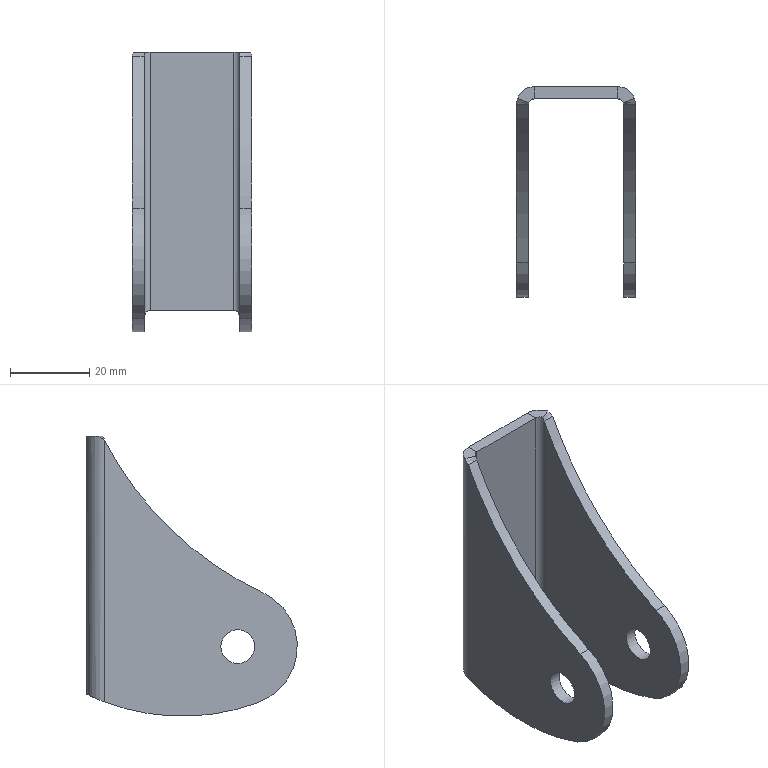Part | STEP file | 6150522 | 1 solid | 26 faces | box 30 x 53 x 70.522 mm | volume 17329 mm3 | cylinder 12 | plane 10 | spline 4 | commonest cylinder face diameters 3 x2 8.5 x2 9 x2 30 x2 110 x2 170 x2
STEP:
#1=CARTESIAN_POINT('',(-15.,-42.25,-11.5));
#2=VERTEX_POINT('',#1);
#3=CARTESIAN_POINT('',(-15.,-38.,-11.5));
#4=DIRECTION('',(-1.,0.,0.));
#5=DIRECTION('',(0.,-1.,0.));
#6=AXIS2_PLACEMENT_3D('',#3,#4,#5);
#7=CIRCLE('',#6,4.25);
#8=EDGE_CURVE('',#2,#2,#7,.T.);
#9=ORIENTED_EDGE('',*,*,#8,.F.);
#10=EDGE_LOOP('',(#9));
#11=FACE_BOUND('',#10,.T.);
#12=CARTESIAN_POINT('',(-15.,-4.5,-25.442));
#13=VERTEX_POINT('',#12);
#14=CARTESIAN_POINT('',(-15.,-4.5,40.505));
#15=VERTEX_POINT('',#14);
#16=CARTESIAN_POINT('',(-15.,-4.5,-41.5));
#17=DIRECTION('',(0.,0.,1.));
#18=VECTOR('',#17,1000.);
#19=LINE('',#16,#18);
#20=EDGE_CURVE('',#13,#15,#19,.T.);
#21=ORIENTED_EDGE('',*,*,#20,.F.);
#22=CARTESIAN_POINT('',(-15.,-43.242,-25.554));
#23=VERTEX_POINT('',#22);
#24=CARTESIAN_POINT('',(-15.,-24.02,25.978));
#25=DIRECTION('',(1.,0.,0.));
#26=DIRECTION('',(0.,-1.,0.));
#27=AXIS2_PLACEMENT_3D('',#24,#25,#26);
#28=CIRCLE('',#27,55.);
#29=EDGE_CURVE('',#23,#13,#28,.T.);
#30=ORIENTED_EDGE('',*,*,#29,.F.);
#31=CARTESIAN_POINT('',(-15.,-44.33,2.099));
#32=VERTEX_POINT('',#31);
#33=CARTESIAN_POINT('',(-15.,-38.,-11.5));
#34=DIRECTION('',(1.,0.,0.));
#35=DIRECTION('',(0.,-1.,0.));
#36=AXIS2_PLACEMENT_3D('',#33,#34,#35);
#37=CIRCLE('',#36,15.);
#38=EDGE_CURVE('',#32,#23,#37,.T.);
#39=ORIENTED_EDGE('',*,*,#38,.F.);
#40=CARTESIAN_POINT('',(-15.,-80.203,79.158));
#41=DIRECTION('',(-1.,0.,0.));
#42=DIRECTION('',(0.,-1.,0.));
#43=AXIS2_PLACEMENT_3D('',#40,#41,#42);
#44=CIRCLE('',#43,85.);
#45=EDGE_CURVE('',#15,#32,#44,.T.);
#46=ORIENTED_EDGE('',*,*,#45,.F.);
#47=EDGE_LOOP('',(#21,#30,#39,#46));
#48=FACE_OUTER_BOUND('',#47,.T.);
#49=CARTESIAN_POINT('',(-15.,0.,-41.5));
#50=DIRECTION('',(-1.,0.,0.));
#51=DIRECTION('',(0.,-1.,0.));
#52=AXIS2_PLACEMENT_3D('',#49,#50,#51);
#53=PLANE('',#52);
#54=ADVANCED_FACE('',(#11,#48),#53,.T.);
#55=CARTESIAN_POINT('',(-10.5,0.,-23.5));
#56=VERTEX_POINT('',#55);
#57=CARTESIAN_POINT('',(-10.5,0.,41.5));
#58=VERTEX_POINT('',#57);
#59=CARTESIAN_POINT('',(-10.5,0.,-41.5));
#60=DIRECTION('',(0.,0.,1.));
#61=VECTOR('',#60,1000.);
#62=LINE('',#59,#61);
#63=EDGE_CURVE('',#56,#58,#62,.T.);
#64=ORIENTED_EDGE('',*,*,#63,.F.);
#65=CARTESIAN_POINT('',(-15.,-4.5,-25.442));
#66=CARTESIAN_POINT('',(-15.,-4.21,-25.332));
#67=CARTESIAN_POINT('',(-14.972,-3.925,-25.221));
#68=CARTESIAN_POINT('',(-14.864,-3.365,-24.997));
#69=CARTESIAN_POINT('',(-14.782,-3.086,-24.884));
#70=CARTESIAN_POINT('',(-14.568,-2.554,-24.661));
#71=CARTESIAN_POINT('',(-14.436,-2.301,-24.553));
#72=CARTESIAN_POINT('',(-14.125,-1.818,-24.343));
#73=CARTESIAN_POINT('',(-13.942,-1.586,-24.24));
#74=CARTESIAN_POINT('',(-13.537,-1.166,-24.05));
#75=CARTESIAN_POINT('',(-13.315,-0.9763,-23.963));
#76=CARTESIAN_POINT('',(-12.828,-0.6378,-23.805));
#77=CARTESIAN_POINT('',(-12.562,-0.4889,-23.735));
#78=CARTESIAN_POINT('',(-12.01,-0.2503,-23.621));
#79=CARTESIAN_POINT('',(-11.722,-0.1583,-23.577));
#80=CARTESIAN_POINT('',(-11.121,-0.03245,-23.516));
#81=CARTESIAN_POINT('',(-10.811,0.,-23.5));
#82=CARTESIAN_POINT('',(-10.5,0.,-23.5));
#83=B_SPLINE_CURVE_WITH_KNOTS('',3,(#65,#66,#67,#68,#69,#70,#71,#72,#73,#74,#75,#76,#77,#78,#79,#80,#81,#82),.UNSPECIFIED.,.F.,.F.,(4,2,2,2,2,2,2,2,4),(0.,0.0009195,0.001839,0.002759,0.003678,0.004598,0.005517,0.006437,0.007356),.UNSPECIFIED.);
#84=EDGE_CURVE('',#13,#56,#83,.T.);
#85=ORIENTED_EDGE('',*,*,#84,.F.);
#86=ORIENTED_EDGE('',*,*,#20,.T.);
#87=CARTESIAN_POINT('',(-14.743,-3.,41.5));
#88=VERTEX_POINT('',#87);
#89=CARTESIAN_POINT('',(-14.743,-3.,41.5));
#90=CARTESIAN_POINT('',(-14.914,-3.484,41.173));
#91=CARTESIAN_POINT('',(-15.,-3.99,40.838));
#92=CARTESIAN_POINT('',(-15.,-4.5,40.505));
#93=B_SPLINE_CURVE_WITH_KNOTS('',3,(#89,#90,#91,#92),.UNSPECIFIED.,.F.,.F.,(4,4),(0.,0.001825),.UNSPECIFIED.);
#94=EDGE_CURVE('',#88,#15,#93,.T.);
#95=ORIENTED_EDGE('',*,*,#94,.F.);
#96=CARTESIAN_POINT('',(-10.5,-4.5,41.5));
#97=DIRECTION('',(0.,0.,1.));
#98=DIRECTION('',(-1.,0.,0.));
#99=AXIS2_PLACEMENT_3D('',#96,#97,#98);
#100=CIRCLE('',#99,4.5);
#101=EDGE_CURVE('',#58,#88,#100,.T.);
#102=ORIENTED_EDGE('',*,*,#101,.F.);
#103=EDGE_LOOP('',(#64,#85,#86,#95,#102));
#104=FACE_OUTER_BOUND('',#103,.T.);
#105=CARTESIAN_POINT('',(-10.5,-4.5,-41.5));
#106=DIRECTION('',(0.,0.,1.));
#107=DIRECTION('',(1.,0.,0.));
#108=AXIS2_PLACEMENT_3D('',#105,#106,#107);
#109=CYLINDRICAL_SURFACE('',#108,4.5);
#110=ADVANCED_FACE('',(#104),#109,.T.);
#111=CARTESIAN_POINT('',(-12.,-4.5,-25.442));
#112=VERTEX_POINT('',#111);
#113=CARTESIAN_POINT('',(-10.5,-3.,-23.5));
#114=VERTEX_POINT('',#113);
#115=CARTESIAN_POINT('',(-12.,-4.5,-25.442));
#116=CARTESIAN_POINT('',(-12.,-4.327,-25.244));
#117=CARTESIAN_POINT('',(-11.971,-4.161,-25.047));
#118=CARTESIAN_POINT('',(-11.859,-3.843,-24.652));
#119=CARTESIAN_POINT('',(-11.775,-3.689,-24.453));
#120=CARTESIAN_POINT('',(-11.545,-3.409,-24.079));
#121=CARTESIAN_POINT('',(-11.398,-3.278,-23.898));
#122=CARTESIAN_POINT('',(-11.108,-3.125,-23.68));
#123=CARTESIAN_POINT('',(-11.,-3.081,-23.617));
#124=CARTESIAN_POINT('',(-10.762,-3.018,-23.526));
#125=CARTESIAN_POINT('',(-10.633,-3.,-23.5));
#126=CARTESIAN_POINT('',(-10.5,-3.,-23.5));
#127=B_SPLINE_CURVE_WITH_KNOTS('',3,(#115,#116,#117,#118,#119,#120,#121,#122,#123,#124,#125,#126),.UNSPECIFIED.,.F.,.F.,(4,2,2,2,2,4),(0.,0.0007778,0.001556,0.002334,0.002722,0.003111),.UNSPECIFIED.);
#128=EDGE_CURVE('',#112,#114,#127,.T.);
#129=ORIENTED_EDGE('',*,*,#128,.T.);
#130=CARTESIAN_POINT('',(-10.5,-3.,41.5));
#131=VERTEX_POINT('',#130);
#132=CARTESIAN_POINT('',(-10.5,-3.,-41.5));
#133=DIRECTION('',(0.,0.,1.));
#134=VECTOR('',#133,1000.);
#135=LINE('',#132,#134);
#136=EDGE_CURVE('',#114,#131,#135,.T.);
#137=ORIENTED_EDGE('',*,*,#136,.T.);
#138=CARTESIAN_POINT('',(-11.914,-4.,41.5));
#139=VERTEX_POINT('',#138);
#140=CARTESIAN_POINT('',(-10.5,-4.5,41.5));
#141=DIRECTION('',(0.,0.,1.));
#142=DIRECTION('',(1.,0.,0.));
#143=AXIS2_PLACEMENT_3D('',#140,#141,#142);
#144=CIRCLE('',#143,1.5);
#145=EDGE_CURVE('',#131,#139,#144,.T.);
#146=ORIENTED_EDGE('',*,*,#145,.T.);
#147=CARTESIAN_POINT('',(-12.,-4.5,40.505));
#148=VERTEX_POINT('',#147);
#149=CARTESIAN_POINT('',(-11.914,-4.,41.5));
#150=CARTESIAN_POINT('',(-11.972,-4.163,41.17));
#151=CARTESIAN_POINT('',(-12.,-4.33,40.837));
#152=CARTESIAN_POINT('',(-12.,-4.5,40.505));
#153=B_SPLINE_CURVE_WITH_KNOTS('',3,(#149,#150,#151,#152),.UNSPECIFIED.,.F.,.F.,(4,4),(0.,0.001118),.UNSPECIFIED.);
#154=EDGE_CURVE('',#139,#148,#153,.T.);
#155=ORIENTED_EDGE('',*,*,#154,.T.);
#156=CARTESIAN_POINT('',(-12.,-4.5,-41.5));
#157=DIRECTION('',(0.,0.,1.));
#158=VECTOR('',#157,1000.);
#159=LINE('',#156,#158);
#160=EDGE_CURVE('',#112,#148,#159,.T.);
#161=ORIENTED_EDGE('',*,*,#160,.F.);
#162=EDGE_LOOP('',(#129,#137,#146,#155,#161));
#163=FACE_OUTER_BOUND('',#162,.T.);
#164=CARTESIAN_POINT('',(-10.5,-4.5,-41.5));
#165=DIRECTION('',(0.,0.,1.));
#166=DIRECTION('',(1.,0.,0.));
#167=AXIS2_PLACEMENT_3D('',#164,#165,#166);
#168=CYLINDRICAL_SURFACE('',#167,1.5);
#169=ADVANCED_FACE('',(#163),#168,.F.);
#170=CARTESIAN_POINT('',(-12.,-42.25,-11.5));
#171=VERTEX_POINT('',#170);
#172=CARTESIAN_POINT('',(-12.,-38.,-11.5));
#173=DIRECTION('',(-1.,0.,0.));
#174=DIRECTION('',(0.,-1.,0.));
#175=AXIS2_PLACEMENT_3D('',#172,#173,#174);
#176=CIRCLE('',#175,4.25);
#177=EDGE_CURVE('',#171,#171,#176,.T.);
#178=ORIENTED_EDGE('',*,*,#177,.T.);
#179=EDGE_LOOP('',(#178));
#180=FACE_BOUND('',#179,.T.);
#181=CARTESIAN_POINT('',(-12.,-43.242,-25.554));
#182=VERTEX_POINT('',#181);
#183=CARTESIAN_POINT('',(-12.,-24.02,25.978));
#184=DIRECTION('',(1.,0.,0.));
#185=DIRECTION('',(0.,-1.,0.));
#186=AXIS2_PLACEMENT_3D('',#183,#184,#185);
#187=CIRCLE('',#186,55.);
#188=EDGE_CURVE('',#182,#112,#187,.T.);
#189=ORIENTED_EDGE('',*,*,#188,.T.);
#190=ORIENTED_EDGE('',*,*,#160,.T.);
#191=CARTESIAN_POINT('',(-12.,-44.33,2.099));
#192=VERTEX_POINT('',#191);
#193=CARTESIAN_POINT('',(-12.,-80.203,79.158));
#194=DIRECTION('',(-1.,0.,0.));
#195=DIRECTION('',(0.,-1.,0.));
#196=AXIS2_PLACEMENT_3D('',#193,#194,#195);
#197=CIRCLE('',#196,85.);
#198=EDGE_CURVE('',#148,#192,#197,.T.);
#199=ORIENTED_EDGE('',*,*,#198,.T.);
#200=CARTESIAN_POINT('',(-12.,-38.,-11.5));
#201=DIRECTION('',(1.,0.,0.));
#202=DIRECTION('',(0.,-1.,0.));
#203=AXIS2_PLACEMENT_3D('',#200,#201,#202);
#204=CIRCLE('',#203,15.);
#205=EDGE_CURVE('',#192,#182,#204,.T.);
#206=ORIENTED_EDGE('',*,*,#205,.T.);
#207=EDGE_LOOP('',(#189,#190,#199,#206));
#208=FACE_OUTER_BOUND('',#207,.T.);
#209=CARTESIAN_POINT('',(-12.,0.,-41.5));
#210=DIRECTION('',(-1.,0.,0.));
#211=DIRECTION('',(0.,-1.,0.));
#212=AXIS2_PLACEMENT_3D('',#209,#210,#211);
#213=PLANE('',#212);
#214=ADVANCED_FACE('',(#180,#208),#213,.F.);
#215=CARTESIAN_POINT('',(15.,-4.5,-25.442));
#216=VERTEX_POINT('',#215);
#217=CARTESIAN_POINT('',(15.,-4.5,40.505));
#218=VERTEX_POINT('',#217);
#219=CARTESIAN_POINT('',(15.,-4.5,-41.5));
#220=DIRECTION('',(0.,0.,1.));
#221=VECTOR('',#220,1000.);
#222=LINE('',#219,#221);
#223=EDGE_CURVE('',#216,#218,#222,.T.);
#224=ORIENTED_EDGE('',*,*,#223,.F.);
#225=CARTESIAN_POINT('',(10.5,0.,-23.5));
#226=VERTEX_POINT('',#225);
#227=CARTESIAN_POINT('',(10.5,0.,-23.5));
#228=CARTESIAN_POINT('',(10.81,0.,-23.5));
#229=CARTESIAN_POINT('',(11.114,-0.03178,-23.515));
#230=CARTESIAN_POINT('',(11.56,-0.124,-23.56));
#231=CARTESIAN_POINT('',(11.707,-0.1622,-23.579));
#232=CARTESIAN_POINT('',(11.998,-0.2538,-23.623));
#233=CARTESIAN_POINT('',(12.142,-0.3074,-23.648));
#234=CARTESIAN_POINT('',(12.558,-0.4869,-23.734));
#235=CARTESIAN_POINT('',(12.819,-0.6322,-23.802));
#236=CARTESIAN_POINT('',(13.309,-0.9719,-23.961));
#237=CARTESIAN_POINT('',(13.535,-1.165,-24.049));
#238=CARTESIAN_POINT('',(13.94,-1.584,-24.239));
#239=CARTESIAN_POINT('',(14.122,-1.814,-24.341));
#240=CARTESIAN_POINT('',(14.436,-2.3,-24.553));
#241=CARTESIAN_POINT('',(14.568,-2.554,-24.661));
#242=CARTESIAN_POINT('',(14.781,-3.084,-24.883));
#243=CARTESIAN_POINT('',(14.863,-3.362,-24.996));
#244=CARTESIAN_POINT('',(14.972,-3.925,-25.221));
#245=CARTESIAN_POINT('',(15.,-4.21,-25.332));
#246=CARTESIAN_POINT('',(15.,-4.5,-25.442));
#247=B_SPLINE_CURVE_WITH_KNOTS('',3,(#227,#228,#229,#230,#231,#232,#233,#234,#235,#236,#237,#238,#239,#240,#241,#242,#243,#244,#245,#246),.UNSPECIFIED.,.F.,.F.,(4,2,2,2,2,2,2,2,2,4),(0.,0.0009144,0.001372,0.001829,0.002743,0.003657,0.004572,0.005486,0.006401,0.007315),.UNSPECIFIED.);
#248=EDGE_CURVE('',#226,#216,#247,.T.);
#249=ORIENTED_EDGE('',*,*,#248,.F.);
#250=CARTESIAN_POINT('',(10.5,0.,41.5));
#251=VERTEX_POINT('',#250);
#252=CARTESIAN_POINT('',(10.5,0.,-41.5));
#253=DIRECTION('',(0.,0.,1.));
#254=VECTOR('',#253,1000.);
#255=LINE('',#252,#254);
#256=EDGE_CURVE('',#226,#251,#255,.T.);
#257=ORIENTED_EDGE('',*,*,#256,.T.);
#258=CARTESIAN_POINT('',(14.743,-3.,41.5));
#259=VERTEX_POINT('',#258);
#260=CARTESIAN_POINT('',(10.5,-4.5,41.5));
#261=DIRECTION('',(0.,0.,1.));
#262=DIRECTION('',(-1.,0.,0.));
#263=AXIS2_PLACEMENT_3D('',#260,#261,#262);
#264=CIRCLE('',#263,4.5);
#265=EDGE_CURVE('',#259,#251,#264,.T.);
#266=ORIENTED_EDGE('',*,*,#265,.F.);
#267=CARTESIAN_POINT('',(15.,-4.5,40.505));
#268=CARTESIAN_POINT('',(15.,-3.99,40.838));
#269=CARTESIAN_POINT('',(14.914,-3.484,41.173));
#270=CARTESIAN_POINT('',(14.743,-3.,41.5));
#271=B_SPLINE_CURVE_WITH_KNOTS('',3,(#267,#268,#269,#270),.UNSPECIFIED.,.F.,.F.,(4,4),(0.,0.001825),.UNSPECIFIED.);
#272=EDGE_CURVE('',#218,#259,#271,.T.);
#273=ORIENTED_EDGE('',*,*,#272,.F.);
#274=EDGE_LOOP('',(#224,#249,#257,#266,#273));
#275=FACE_OUTER_BOUND('',#274,.T.);
#276=CARTESIAN_POINT('',(10.5,-4.5,-41.5));
#277=DIRECTION('',(0.,0.,1.));
#278=DIRECTION('',(1.,0.,0.));
#279=AXIS2_PLACEMENT_3D('',#276,#277,#278);
#280=CYLINDRICAL_SURFACE('',#279,4.5);
#281=ADVANCED_FACE('',(#275),#280,.T.);
#282=CARTESIAN_POINT('',(15.,-33.75,-11.5));
#283=VERTEX_POINT('',#282);
#284=CARTESIAN_POINT('',(15.,-38.,-11.5));
#285=DIRECTION('',(1.,0.,0.));
#286=DIRECTION('',(0.,1.,0.));
#287=AXIS2_PLACEMENT_3D('',#284,#285,#286);
#288=CIRCLE('',#287,4.25);
#289=EDGE_CURVE('',#283,#283,#288,.T.);
#290=ORIENTED_EDGE('',*,*,#289,.F.);
#291=EDGE_LOOP('',(#290));
#292=FACE_BOUND('',#291,.T.);
#293=CARTESIAN_POINT('',(15.,-43.242,-25.554));
#294=VERTEX_POINT('',#293);
#295=CARTESIAN_POINT('',(15.,-44.33,2.099));
#296=VERTEX_POINT('',#295);
#297=CARTESIAN_POINT('',(15.,-38.,-11.5));
#298=DIRECTION('',(-1.,0.,0.));
#299=DIRECTION('',(0.,1.,0.));
#300=AXIS2_PLACEMENT_3D('',#297,#298,#299);
#301=CIRCLE('',#300,15.);
#302=EDGE_CURVE('',#294,#296,#301,.T.);
#303=ORIENTED_EDGE('',*,*,#302,.F.);
#304=CARTESIAN_POINT('',(15.,-24.02,25.978));
#305=DIRECTION('',(-1.,0.,0.));
#306=DIRECTION('',(0.,1.,0.));
#307=AXIS2_PLACEMENT_3D('',#304,#305,#306);
#308=CIRCLE('',#307,55.);
#309=EDGE_CURVE('',#216,#294,#308,.T.);
#310=ORIENTED_EDGE('',*,*,#309,.F.);
#311=ORIENTED_EDGE('',*,*,#223,.T.);
#312=CARTESIAN_POINT('',(15.,-80.203,79.158));
#313=DIRECTION('',(1.,0.,0.));
#314=DIRECTION('',(0.,1.,0.));
#315=AXIS2_PLACEMENT_3D('',#312,#313,#314);
#316=CIRCLE('',#315,85.);
#317=EDGE_CURVE('',#296,#218,#316,.T.);
#318=ORIENTED_EDGE('',*,*,#317,.F.);
#319=EDGE_LOOP('',(#303,#310,#311,#318));
#320=FACE_OUTER_BOUND('',#319,.T.);
#321=CARTESIAN_POINT('',(15.,0.,-41.5));
#322=DIRECTION('',(1.,0.,0.));
#323=DIRECTION('',(0.,1.,0.));
#324=AXIS2_PLACEMENT_3D('',#321,#322,#323);
#325=PLANE('',#324);
#326=ADVANCED_FACE('',(#292,#320),#325,.T.);
#327=CARTESIAN_POINT('',(12.,-33.75,-11.5));
#328=VERTEX_POINT('',#327);
#329=CARTESIAN_POINT('',(12.,-38.,-11.5));
#330=DIRECTION('',(1.,0.,0.));
#331=DIRECTION('',(0.,1.,0.));
#332=AXIS2_PLACEMENT_3D('',#329,#330,#331);
#333=CIRCLE('',#332,4.25);
#334=EDGE_CURVE('',#328,#328,#333,.T.);
#335=ORIENTED_EDGE('',*,*,#334,.T.);
#336=EDGE_LOOP('',(#335));
#337=FACE_BOUND('',#336,.T.);
#338=CARTESIAN_POINT('',(12.,-4.5,-25.442));
#339=VERTEX_POINT('',#338);
#340=CARTESIAN_POINT('',(12.,-43.242,-25.554));
#341=VERTEX_POINT('',#340);
#342=CARTESIAN_POINT('',(12.,-24.02,25.978));
#343=DIRECTION('',(-1.,0.,0.));
#344=DIRECTION('',(0.,1.,0.));
#345=AXIS2_PLACEMENT_3D('',#342,#343,#344);
#346=CIRCLE('',#345,55.);
#347=EDGE_CURVE('',#339,#341,#346,.T.);
#348=ORIENTED_EDGE('',*,*,#347,.T.);
#349=CARTESIAN_POINT('',(12.,-44.33,2.099));
#350=VERTEX_POINT('',#349);
#351=CARTESIAN_POINT('',(12.,-38.,-11.5));
#352=DIRECTION('',(-1.,0.,0.));
#353=DIRECTION('',(0.,1.,0.));
#354=AXIS2_PLACEMENT_3D('',#351,#352,#353);
#355=CIRCLE('',#354,15.);
#356=EDGE_CURVE('',#341,#350,#355,.T.);
#357=ORIENTED_EDGE('',*,*,#356,.T.);
#358=CARTESIAN_POINT('',(12.,-4.5,40.505));
#359=VERTEX_POINT('',#358);
#360=CARTESIAN_POINT('',(12.,-80.203,79.158));
#361=DIRECTION('',(1.,0.,0.));
#362=DIRECTION('',(0.,1.,0.));
#363=AXIS2_PLACEMENT_3D('',#360,#361,#362);
#364=CIRCLE('',#363,85.);
#365=EDGE_CURVE('',#350,#359,#364,.T.);
#366=ORIENTED_EDGE('',*,*,#365,.T.);
#367=CARTESIAN_POINT('',(12.,-4.5,-41.5));
#368=DIRECTION('',(0.,0.,1.));
#369=VECTOR('',#368,1000.);
#370=LINE('',#367,#369);
#371=EDGE_CURVE('',#339,#359,#370,.T.);
#372=ORIENTED_EDGE('',*,*,#371,.F.);
#373=EDGE_LOOP('',(#348,#357,#366,#372));
#374=FACE_OUTER_BOUND('',#373,.T.);
#375=CARTESIAN_POINT('',(12.,0.,-41.5));
#376=DIRECTION('',(1.,0.,0.));
#377=DIRECTION('',(0.,1.,0.));
#378=AXIS2_PLACEMENT_3D('',#375,#376,#377);
#379=PLANE('',#378);
#380=ADVANCED_FACE('',(#337,#374),#379,.F.);
#381=CARTESIAN_POINT('',(10.5,-3.,-23.5));
#382=VERTEX_POINT('',#381);
#383=CARTESIAN_POINT('',(10.5,-3.,-23.5));
#384=CARTESIAN_POINT('',(10.633,-3.,-23.5));
#385=CARTESIAN_POINT('',(10.762,-3.018,-23.526));
#386=CARTESIAN_POINT('',(11.001,-3.081,-23.617));
#387=CARTESIAN_POINT('',(11.109,-3.125,-23.681));
#388=CARTESIAN_POINT('',(11.397,-3.279,-23.898));
#389=CARTESIAN_POINT('',(11.545,-3.409,-24.079));
#390=CARTESIAN_POINT('',(11.774,-3.688,-24.453));
#391=CARTESIAN_POINT('',(11.858,-3.842,-24.651));
#392=CARTESIAN_POINT('',(11.971,-4.161,-25.047));
#393=CARTESIAN_POINT('',(12.,-4.327,-25.245));
#394=CARTESIAN_POINT('',(12.,-4.5,-25.442));
#395=B_SPLINE_CURVE_WITH_KNOTS('',3,(#383,#384,#385,#386,#387,#388,#389,#390,#391,#392,#393,#394),.UNSPECIFIED.,.F.,.F.,(4,2,2,2,2,4),(0.,0.0003916,0.0007832,0.001566,0.00235,0.003133),.UNSPECIFIED.);
#396=EDGE_CURVE('',#382,#339,#395,.T.);
#397=ORIENTED_EDGE('',*,*,#396,.T.);
#398=ORIENTED_EDGE('',*,*,#371,.T.);
#399=CARTESIAN_POINT('',(11.914,-4.,41.5));
#400=VERTEX_POINT('',#399);
#401=CARTESIAN_POINT('',(12.,-4.5,40.505));
#402=CARTESIAN_POINT('',(12.,-4.443,40.616));
#403=CARTESIAN_POINT('',(11.997,-4.387,40.728));
#404=CARTESIAN_POINT('',(11.99,-4.33,40.839));
#405=CARTESIAN_POINT('',(11.984,-4.275,40.949));
#406=CARTESIAN_POINT('',(11.975,-4.219,41.06));
#407=CARTESIAN_POINT('',(11.962,-4.164,41.17));
#408=CARTESIAN_POINT('',(11.949,-4.109,41.28));
#409=CARTESIAN_POINT('',(11.933,-4.054,41.39));
#410=CARTESIAN_POINT('',(11.914,-4.,41.5));
#411=B_SPLINE_CURVE_WITH_KNOTS('',3,(#401,#402,#403,#404,#405,#406,#407,#408,#409,#410),.UNSPECIFIED.,.F.,.F.,(4,3,3,4),(0.,0.0003751,0.0007461,0.001118),.UNSPECIFIED.);
#412=EDGE_CURVE('',#359,#400,#411,.T.);
#413=ORIENTED_EDGE('',*,*,#412,.T.);
#414=CARTESIAN_POINT('',(10.5,-3.,41.5));
#415=VERTEX_POINT('',#414);
#416=CARTESIAN_POINT('',(10.5,-4.5,41.5));
#417=DIRECTION('',(0.,0.,1.));
#418=DIRECTION('',(1.,0.,0.));
#419=AXIS2_PLACEMENT_3D('',#416,#417,#418);
#420=CIRCLE('',#419,1.5);
#421=EDGE_CURVE('',#400,#415,#420,.T.);
#422=ORIENTED_EDGE('',*,*,#421,.T.);
#423=CARTESIAN_POINT('',(10.5,-3.,-41.5));
#424=DIRECTION('',(0.,0.,1.));
#425=VECTOR('',#424,1000.);
#426=LINE('',#423,#425);
#427=EDGE_CURVE('',#382,#415,#426,.T.);
#428=ORIENTED_EDGE('',*,*,#427,.F.);
#429=EDGE_LOOP('',(#397,#398,#413,#422,#428));
#430=FACE_OUTER_BOUND('',#429,.T.);
#431=CARTESIAN_POINT('',(10.5,-4.5,-41.5));
#432=DIRECTION('',(0.,0.,1.));
#433=DIRECTION('',(1.,0.,0.));
#434=AXIS2_PLACEMENT_3D('',#431,#432,#433);
#435=CYLINDRICAL_SURFACE('',#434,1.5);
#436=ADVANCED_FACE('',(#430),#435,.F.);
#437=ORIENTED_EDGE('',*,*,#256,.F.);
#438=CARTESIAN_POINT('',(141.808,0.,-23.5));
#439=DIRECTION('',(-1.,0.,0.));
#440=VECTOR('',#439,1000.);
#441=LINE('',#438,#440);
#442=EDGE_CURVE('',#226,#56,#441,.T.);
#443=ORIENTED_EDGE('',*,*,#442,.T.);
#444=ORIENTED_EDGE('',*,*,#63,.T.);
#445=CARTESIAN_POINT('',(-15.,0.,41.5));
#446=DIRECTION('',(-1.,0.,0.));
#447=VECTOR('',#446,1000.);
#448=LINE('',#445,#447);
#449=EDGE_CURVE('',#251,#58,#448,.T.);
#450=ORIENTED_EDGE('',*,*,#449,.F.);
#451=EDGE_LOOP('',(#437,#443,#444,#450));
#452=FACE_OUTER_BOUND('',#451,.T.);
#453=CARTESIAN_POINT('',(-15.,0.,-41.5));
#454=DIRECTION('',(0.,1.,0.));
#455=DIRECTION('',(0.,0.,1.));
#456=AXIS2_PLACEMENT_3D('',#453,#454,#455);
#457=PLANE('',#456);
#458=ADVANCED_FACE('',(#452),#457,.T.);
#459=CARTESIAN_POINT('',(-15.,-3.,-23.5));
#460=DIRECTION('',(-1.,0.,0.));
#461=VECTOR('',#460,1000.);
#462=LINE('',#459,#461);
#463=EDGE_CURVE('',#382,#114,#462,.T.);
#464=ORIENTED_EDGE('',*,*,#463,.F.);
#465=ORIENTED_EDGE('',*,*,#427,.T.);
#466=CARTESIAN_POINT('',(-15.,-3.,41.5));
#467=DIRECTION('',(-1.,0.,0.));
#468=VECTOR('',#467,1000.);
#469=LINE('',#466,#468);
#470=EDGE_CURVE('',#415,#131,#469,.T.);
#471=ORIENTED_EDGE('',*,*,#470,.T.);
#472=ORIENTED_EDGE('',*,*,#136,.F.);
#473=EDGE_LOOP('',(#464,#465,#471,#472));
#474=FACE_OUTER_BOUND('',#473,.T.);
#475=CARTESIAN_POINT('',(-15.,-3.,-41.5));
#476=DIRECTION('',(0.,1.,0.));
#477=DIRECTION('',(0.,0.,1.));
#478=AXIS2_PLACEMENT_3D('',#475,#476,#477);
#479=PLANE('',#478);
#480=ADVANCED_FACE('',(#474),#479,.F.);
#481=ORIENTED_EDGE('',*,*,#101,.T.);
#482=CARTESIAN_POINT('',(-14.743,-3.,41.5));
#483=DIRECTION('',(-0.9428,0.3333,0.));
#484=VECTOR('',#483,1000.);
#485=LINE('',#482,#484);
#486=EDGE_CURVE('',#139,#88,#485,.T.);
#487=ORIENTED_EDGE('',*,*,#486,.F.);
#488=ORIENTED_EDGE('',*,*,#145,.F.);
#489=CARTESIAN_POINT('',(-10.5,0.,41.5));
#490=DIRECTION('',(0.,-1.,0.));
#491=VECTOR('',#490,1000.);
#492=LINE('',#489,#491);
#493=EDGE_CURVE('',#58,#131,#492,.T.);
#494=ORIENTED_EDGE('',*,*,#493,.F.);
#495=EDGE_LOOP('',(#481,#487,#488,#494));
#496=FACE_OUTER_BOUND('',#495,.T.);
#497=CARTESIAN_POINT('',(-10.5,0.,41.5));
#498=DIRECTION('',(0.,0.,1.));
#499=DIRECTION('',(1.,0.,0.));
#500=AXIS2_PLACEMENT_3D('',#497,#498,#499);
#501=PLANE('',#500);
#502=ADVANCED_FACE('',(#496),#501,.T.);
#503=ORIENTED_EDGE('',*,*,#421,.F.);
#504=CARTESIAN_POINT('',(11.914,-4.,41.5));
#505=DIRECTION('',(0.9428,0.3333,0.));
#506=VECTOR('',#505,1000.);
#507=LINE('',#504,#506);
#508=EDGE_CURVE('',#400,#259,#507,.T.);
#509=ORIENTED_EDGE('',*,*,#508,.T.);
#510=ORIENTED_EDGE('',*,*,#265,.T.);
#511=CARTESIAN_POINT('',(10.5,-3.,41.5));
#512=DIRECTION('',(0.,1.,0.));
#513=VECTOR('',#512,1000.);
#514=LINE('',#511,#513);
#515=EDGE_CURVE('',#415,#251,#514,.T.);
#516=ORIENTED_EDGE('',*,*,#515,.F.);
#517=EDGE_LOOP('',(#503,#509,#510,#516));
#518=FACE_OUTER_BOUND('',#517,.T.);
#519=CARTESIAN_POINT('',(15.,-4.5,41.5));
#520=DIRECTION('',(0.,0.,1.));
#521=DIRECTION('',(1.,0.,0.));
#522=AXIS2_PLACEMENT_3D('',#519,#520,#521);
#523=PLANE('',#522);
#524=ADVANCED_FACE('',(#518),#523,.T.);
#525=ORIENTED_EDGE('',*,*,#449,.T.);
#526=ORIENTED_EDGE('',*,*,#493,.T.);
#527=ORIENTED_EDGE('',*,*,#470,.F.);
#528=ORIENTED_EDGE('',*,*,#515,.T.);
#529=EDGE_LOOP('',(#525,#526,#527,#528));
#530=FACE_OUTER_BOUND('',#529,.T.);
#531=CARTESIAN_POINT('',(-12.,-4.5,41.5));
#532=DIRECTION('',(0.,0.,1.));
#533=DIRECTION('',(1.,0.,0.));
#534=AXIS2_PLACEMENT_3D('',#531,#532,#533);
#535=PLANE('',#534);
#536=ADVANCED_FACE('',(#530),#535,.T.);
#537=ORIENTED_EDGE('',*,*,#356,.F.);
#538=CARTESIAN_POINT('',(12.,-43.242,-25.554));
#539=DIRECTION('',(1.,0.,0.));
#540=VECTOR('',#539,1000.);
#541=LINE('',#538,#540);
#542=EDGE_CURVE('',#341,#294,#541,.T.);
#543=ORIENTED_EDGE('',*,*,#542,.T.);
#544=ORIENTED_EDGE('',*,*,#302,.T.);
#545=CARTESIAN_POINT('',(15.,-44.33,2.099));
#546=DIRECTION('',(-1.,0.,0.));
#547=VECTOR('',#546,1000.);
#548=LINE('',#545,#547);
#549=EDGE_CURVE('',#296,#350,#548,.T.);
#550=ORIENTED_EDGE('',*,*,#549,.T.);
#551=EDGE_LOOP('',(#537,#543,#544,#550));
#552=FACE_OUTER_BOUND('',#551,.T.);
#553=CARTESIAN_POINT('',(15.,-38.,-11.5));
#554=DIRECTION('',(1.,0.,0.));
#555=DIRECTION('',(0.,1.,0.));
#556=AXIS2_PLACEMENT_3D('',#553,#554,#555);
#557=CYLINDRICAL_SURFACE('',#556,15.);
#558=ADVANCED_FACE('',(#552),#557,.T.);
#559=ORIENTED_EDGE('',*,*,#317,.T.);
#560=CARTESIAN_POINT('',(15.,-4.5,40.505));
#561=DIRECTION('',(-1.,0.,0.));
#562=VECTOR('',#561,1000.);
#563=LINE('',#560,#562);
#564=EDGE_CURVE('',#218,#359,#563,.T.);
#565=ORIENTED_EDGE('',*,*,#564,.T.);
#566=ORIENTED_EDGE('',*,*,#365,.F.);
#567=ORIENTED_EDGE('',*,*,#549,.F.);
#568=EDGE_LOOP('',(#559,#565,#566,#567));
#569=FACE_OUTER_BOUND('',#568,.T.);
#570=CARTESIAN_POINT('',(15.,-80.203,79.158));
#571=DIRECTION('',(1.,0.,0.));
#572=DIRECTION('',(0.,1.,0.));
#573=AXIS2_PLACEMENT_3D('',#570,#571,#572);
#574=CYLINDRICAL_SURFACE('',#573,85.);
#575=ADVANCED_FACE('',(#569),#574,.F.);
#576=ORIENTED_EDGE('',*,*,#508,.F.);
#577=ORIENTED_EDGE('',*,*,#412,.F.);
#578=ORIENTED_EDGE('',*,*,#564,.F.);
#579=ORIENTED_EDGE('',*,*,#272,.T.);
#580=EDGE_LOOP('',(#576,#577,#578,#579));
#581=FACE_OUTER_BOUND('',#580,.T.);
#582=CARTESIAN_POINT('',(11.97,-4.5,40.505));
#583=CARTESIAN_POINT('',(11.97,-4.334,40.837));
#584=CARTESIAN_POINT('',(11.943,-4.17,41.169));
#585=CARTESIAN_POINT('',(11.886,-4.01,41.5));
#586=CARTESIAN_POINT('',(12.,-4.5,40.505));
#587=CARTESIAN_POINT('',(12.,-4.33,40.837));
#588=CARTESIAN_POINT('',(11.972,-4.163,41.169));
#589=CARTESIAN_POINT('',(11.914,-4.,41.5));
#590=CARTESIAN_POINT('',(15.,-4.5,40.505));
#591=CARTESIAN_POINT('',(15.,-3.991,40.837));
#592=CARTESIAN_POINT('',(14.916,-3.49,41.169));
#593=CARTESIAN_POINT('',(14.743,-3.,41.5));
#594=B_SPLINE_SURFACE_WITH_KNOTS('',1,3,((#582,#583,#584,#585),(#586,#587,#588,#589),(#590,#591,#592,#593)),.UNSPECIFIED.,.F.,.F.,.F.,(2,1,2),(4,4),(-0.01,0.,1.),(0.,0.001117),.UNSPECIFIED.);
#595=ADVANCED_FACE('',(#581),#594,.T.);
#596=CARTESIAN_POINT('',(-15.,-44.33,2.099));
#597=DIRECTION('',(1.,0.,0.));
#598=VECTOR('',#597,1000.);
#599=LINE('',#596,#598);
#600=EDGE_CURVE('',#32,#192,#599,.T.);
#601=ORIENTED_EDGE('',*,*,#600,.F.);
#602=ORIENTED_EDGE('',*,*,#38,.T.);
#603=CARTESIAN_POINT('',(-12.,-43.242,-25.554));
#604=DIRECTION('',(-1.,0.,0.));
#605=VECTOR('',#604,1000.);
#606=LINE('',#603,#605);
#607=EDGE_CURVE('',#182,#23,#606,.T.);
#608=ORIENTED_EDGE('',*,*,#607,.F.);
#609=ORIENTED_EDGE('',*,*,#205,.F.);
#610=EDGE_LOOP('',(#601,#602,#608,#609));
#611=FACE_OUTER_BOUND('',#610,.T.);
#612=CARTESIAN_POINT('',(-15.,-38.,-11.5));
#613=DIRECTION('',(-1.,0.,0.));
#614=DIRECTION('',(0.,-1.,0.));
#615=AXIS2_PLACEMENT_3D('',#612,#613,#614);
#616=CYLINDRICAL_SURFACE('',#615,15.);
#617=ADVANCED_FACE('',(#611),#616,.T.);
#618=ORIENTED_EDGE('',*,*,#45,.T.);
#619=ORIENTED_EDGE('',*,*,#600,.T.);
#620=ORIENTED_EDGE('',*,*,#198,.F.);
#621=CARTESIAN_POINT('',(-15.,-4.5,40.505));
#622=DIRECTION('',(1.,0.,0.));
#623=VECTOR('',#622,1000.);
#624=LINE('',#621,#623);
#625=EDGE_CURVE('',#15,#148,#624,.T.);
#626=ORIENTED_EDGE('',*,*,#625,.F.);
#627=EDGE_LOOP('',(#618,#619,#620,#626));
#628=FACE_OUTER_BOUND('',#627,.T.);
#629=CARTESIAN_POINT('',(-15.,-80.203,79.158));
#630=DIRECTION('',(-1.,0.,0.));
#631=DIRECTION('',(0.,-1.,0.));
#632=AXIS2_PLACEMENT_3D('',#629,#630,#631);
#633=CYLINDRICAL_SURFACE('',#632,85.);
#634=ADVANCED_FACE('',(#628),#633,.F.);
#635=ORIENTED_EDGE('',*,*,#625,.T.);
#636=ORIENTED_EDGE('',*,*,#154,.F.);
#637=ORIENTED_EDGE('',*,*,#486,.T.);
#638=ORIENTED_EDGE('',*,*,#94,.T.);
#639=EDGE_LOOP('',(#635,#636,#637,#638));
#640=FACE_OUTER_BOUND('',#639,.T.);
#641=CARTESIAN_POINT('',(-11.886,-4.01,41.5));
#642=CARTESIAN_POINT('',(-11.943,-4.17,41.169));
#643=CARTESIAN_POINT('',(-11.97,-4.334,40.837));
#644=CARTESIAN_POINT('',(-11.97,-4.5,40.505));
#645=CARTESIAN_POINT('',(-11.914,-4.,41.5));
#646=CARTESIAN_POINT('',(-11.972,-4.163,41.169));
#647=CARTESIAN_POINT('',(-12.,-4.33,40.837));
#648=CARTESIAN_POINT('',(-12.,-4.5,40.505));
#649=CARTESIAN_POINT('',(-14.743,-3.,41.5));
#650=CARTESIAN_POINT('',(-14.916,-3.49,41.169));
#651=CARTESIAN_POINT('',(-15.,-3.991,40.837));
#652=CARTESIAN_POINT('',(-15.,-4.5,40.505));
#653=B_SPLINE_SURFACE_WITH_KNOTS('',1,3,((#641,#642,#643,#644),(#645,#646,#647,#648),(#649,#650,#651,#652)),.UNSPECIFIED.,.F.,.F.,.F.,(2,1,2),(4,4),(-0.01,0.,1.),(0.,0.001117),.UNSPECIFIED.);
#654=ADVANCED_FACE('',(#640),#653,.T.);
#655=CARTESIAN_POINT('',(-12.,-4.5,-25.442));
#656=DIRECTION('',(-1.,0.,0.));
#657=VECTOR('',#656,1000.);
#658=LINE('',#655,#657);
#659=EDGE_CURVE('',#112,#13,#658,.T.);
#660=ORIENTED_EDGE('',*,*,#659,.F.);
#661=ORIENTED_EDGE('',*,*,#188,.F.);
#662=ORIENTED_EDGE('',*,*,#607,.T.);
#663=ORIENTED_EDGE('',*,*,#29,.T.);
#664=EDGE_LOOP('',(#660,#661,#662,#663));
#665=FACE_OUTER_BOUND('',#664,.T.);
#666=CARTESIAN_POINT('',(-12.,-24.02,25.978));
#667=DIRECTION('',(-1.,0.,0.));
#668=DIRECTION('',(0.,-1.,0.));
#669=AXIS2_PLACEMENT_3D('',#666,#667,#668);
#670=CYLINDRICAL_SURFACE('',#669,55.);
#671=ADVANCED_FACE('',(#665),#670,.T.);
#672=ORIENTED_EDGE('',*,*,#442,.F.);
#673=CARTESIAN_POINT('',(10.5,0.,-23.5));
#674=DIRECTION('',(0.,-1.,0.));
#675=VECTOR('',#674,1000.);
#676=LINE('',#673,#675);
#677=EDGE_CURVE('',#226,#382,#676,.T.);
#678=ORIENTED_EDGE('',*,*,#677,.T.);
#679=ORIENTED_EDGE('',*,*,#463,.T.);
#680=CARTESIAN_POINT('',(-10.5,0.,-23.5));
#681=DIRECTION('',(0.,-1.,0.));
#682=VECTOR('',#681,1000.);
#683=LINE('',#680,#682);
#684=EDGE_CURVE('',#56,#114,#683,.T.);
#685=ORIENTED_EDGE('',*,*,#684,.F.);
#686=EDGE_LOOP('',(#672,#678,#679,#685));
#687=FACE_OUTER_BOUND('',#686,.T.);
#688=CARTESIAN_POINT('',(141.808,0.,-23.5));
#689=DIRECTION('',(0.,0.,-1.));
#690=DIRECTION('',(-1.,0.,0.));
#691=AXIS2_PLACEMENT_3D('',#688,#689,#690);
#692=PLANE('',#691);
#693=ADVANCED_FACE('',(#687),#692,.T.);
#694=ORIENTED_EDGE('',*,*,#542,.F.);
#695=ORIENTED_EDGE('',*,*,#347,.F.);
#696=CARTESIAN_POINT('',(12.,-4.5,-25.442));
#697=DIRECTION('',(1.,0.,0.));
#698=VECTOR('',#697,1000.);
#699=LINE('',#696,#698);
#700=EDGE_CURVE('',#339,#216,#699,.T.);
#701=ORIENTED_EDGE('',*,*,#700,.T.);
#702=ORIENTED_EDGE('',*,*,#309,.T.);
#703=EDGE_LOOP('',(#694,#695,#701,#702));
#704=FACE_OUTER_BOUND('',#703,.T.);
#705=CARTESIAN_POINT('',(12.,-24.02,25.978));
#706=DIRECTION('',(1.,0.,0.));
#707=DIRECTION('',(0.,1.,0.));
#708=AXIS2_PLACEMENT_3D('',#705,#706,#707);
#709=CYLINDRICAL_SURFACE('',#708,55.);
#710=ADVANCED_FACE('',(#704),#709,.T.);
#711=ORIENTED_EDGE('',*,*,#248,.T.);
#712=ORIENTED_EDGE('',*,*,#700,.F.);
#713=ORIENTED_EDGE('',*,*,#396,.F.);
#714=ORIENTED_EDGE('',*,*,#677,.F.);
#715=EDGE_LOOP('',(#711,#712,#713,#714));
#716=FACE_OUTER_BOUND('',#715,.T.);
#717=CARTESIAN_POINT('',(10.5,-3.03,-23.5));
#718=CARTESIAN_POINT('',(10.601,-3.03,-23.5));
#719=CARTESIAN_POINT('',(10.701,-3.04,-23.515));
#720=CARTESIAN_POINT('',(10.896,-3.081,-23.575));
#721=CARTESIAN_POINT('',(10.992,-3.111,-23.62));
#722=CARTESIAN_POINT('',(11.263,-3.228,-23.791));
#723=CARTESIAN_POINT('',(11.426,-3.342,-23.955));
#724=CARTESIAN_POINT('',(11.624,-3.548,-24.239));
#725=CARTESIAN_POINT('',(11.684,-3.623,-24.342));
#726=CARTESIAN_POINT('',(11.786,-3.782,-24.553));
#727=CARTESIAN_POINT('',(11.829,-3.865,-24.662));
#728=CARTESIAN_POINT('',(11.899,-4.038,-24.884));
#729=CARTESIAN_POINT('',(11.925,-4.129,-24.997));
#730=CARTESIAN_POINT('',(11.961,-4.312,-25.221));
#731=CARTESIAN_POINT('',(11.97,-4.405,-25.332));
#732=CARTESIAN_POINT('',(11.97,-4.5,-25.442));
#733=CARTESIAN_POINT('',(10.5,-3.,-23.5));
#734=CARTESIAN_POINT('',(10.603,-3.,-23.5));
#735=CARTESIAN_POINT('',(10.705,-3.011,-23.515));
#736=CARTESIAN_POINT('',(10.904,-3.052,-23.575));
#737=CARTESIAN_POINT('',(11.002,-3.083,-23.62));
#738=CARTESIAN_POINT('',(11.279,-3.202,-23.791));
#739=CARTESIAN_POINT('',(11.445,-3.319,-23.955));
#740=CARTESIAN_POINT('',(11.647,-3.529,-24.239));
#741=CARTESIAN_POINT('',(11.708,-3.605,-24.342));
#742=CARTESIAN_POINT('',(11.812,-3.767,-24.553));
#743=CARTESIAN_POINT('',(11.856,-3.852,-24.662));
#744=CARTESIAN_POINT('',(11.927,-4.029,-24.884));
#745=CARTESIAN_POINT('',(11.955,-4.122,-24.997));
#746=CARTESIAN_POINT('',(11.991,-4.309,-25.221));
#747=CARTESIAN_POINT('',(12.,-4.403,-25.332));
#748=CARTESIAN_POINT('',(12.,-4.5,-25.442));
#749=CARTESIAN_POINT('',(10.5,0.,-23.5));
#750=CARTESIAN_POINT('',(10.81,0.,-23.5));
#751=CARTESIAN_POINT('',(11.115,-0.03176,-23.515));
#752=CARTESIAN_POINT('',(11.711,-0.1554,-23.575));
#753=CARTESIAN_POINT('',(12.007,-0.249,-23.62));
#754=CARTESIAN_POINT('',(12.837,-0.6073,-23.791));
#755=CARTESIAN_POINT('',(13.334,-0.9564,-23.955));
#756=CARTESIAN_POINT('',(13.941,-1.586,-24.239));
#757=CARTESIAN_POINT('',(14.124,-1.816,-24.342));
#758=CARTESIAN_POINT('',(14.437,-2.301,-24.553));
#759=CARTESIAN_POINT('',(14.568,-2.555,-24.662));
#760=CARTESIAN_POINT('',(14.782,-3.086,-24.884));
#761=CARTESIAN_POINT('',(14.864,-3.365,-24.997));
#762=CARTESIAN_POINT('',(14.972,-3.926,-25.221));
#763=CARTESIAN_POINT('',(15.,-4.21,-25.332));
#764=CARTESIAN_POINT('',(15.,-4.5,-25.442));
#765=CARTESIAN_POINT('',(10.5,0.0303,-23.5));
#766=CARTESIAN_POINT('',(10.812,0.0303,-23.5));
#767=CARTESIAN_POINT('',(11.119,-0.001677,-23.515));
#768=CARTESIAN_POINT('',(11.719,-0.1261,-23.575));
#769=CARTESIAN_POINT('',(12.017,-0.2204,-23.62));
#770=CARTESIAN_POINT('',(12.852,-0.5811,-23.791));
#771=CARTESIAN_POINT('',(13.353,-0.9326,-23.955));
#772=CARTESIAN_POINT('',(13.964,-1.566,-24.239));
#773=CARTESIAN_POINT('',(14.148,-1.798,-24.342));
#774=CARTESIAN_POINT('',(14.463,-2.286,-24.553));
#775=CARTESIAN_POINT('',(14.595,-2.542,-24.662));
#776=CARTESIAN_POINT('',(14.811,-3.077,-24.884));
#777=CARTESIAN_POINT('',(14.893,-3.357,-24.997));
#778=CARTESIAN_POINT('',(15.002,-3.922,-25.221));
#779=CARTESIAN_POINT('',(15.03,-4.208,-25.332));
#780=CARTESIAN_POINT('',(15.03,-4.5,-25.442));
#781=B_SPLINE_SURFACE_WITH_KNOTS('',1,3,((#717,#718,#719,#720,#721,#722,#723,#724,#725,#726,#727,#728,#729,#730,#731,#732),(#733,#734,#735,#736,#737,#738,#739,#740,#741,#742,#743,#744,#745,#746,#747,#748),(#749,#750,#751,#752,#753,#754,#755,#756,#757,#758,#759,#760,#761,#762,#763,#764),(#765,#766,#767,#768,#769,#770,#771,#772,#773,#774,#775,#776,#777,#778,#779,#780)),.UNSPECIFIED.,.F.,.F.,.F.,(2,1,1,2),(4,2,2,2,2,2,2,4),(-0.01,0.,1.,1.01),(0.,0.0009172,0.001834,0.003669,0.004586,0.005503,0.00642,0.007337),.UNSPECIFIED.);
#782=ADVANCED_FACE('',(#716),#781,.T.);
#783=ORIENTED_EDGE('',*,*,#84,.T.);
#784=ORIENTED_EDGE('',*,*,#684,.T.);
#785=ORIENTED_EDGE('',*,*,#128,.F.);
#786=ORIENTED_EDGE('',*,*,#659,.T.);
#787=EDGE_LOOP('',(#783,#784,#785,#786));
#788=FACE_OUTER_BOUND('',#787,.T.);
#789=CARTESIAN_POINT('',(-11.97,-4.5,-25.442));
#790=CARTESIAN_POINT('',(-11.97,-4.311,-25.223));
#791=CARTESIAN_POINT('',(-11.934,-4.127,-24.997));
#792=CARTESIAN_POINT('',(-11.829,-3.865,-24.662));
#793=CARTESIAN_POINT('',(-11.786,-3.782,-24.553));
#794=CARTESIAN_POINT('',(-11.684,-3.624,-24.343));
#795=CARTESIAN_POINT('',(-11.625,-3.549,-24.241));
#796=CARTESIAN_POINT('',(-11.492,-3.411,-24.05));
#797=CARTESIAN_POINT('',(-11.419,-3.349,-23.962));
#798=CARTESIAN_POINT('',(-11.261,-3.239,-23.805));
#799=CARTESIAN_POINT('',(-11.174,-3.19,-23.735));
#800=CARTESIAN_POINT('',(-10.902,-3.072,-23.564));
#801=CARTESIAN_POINT('',(-10.705,-3.03,-23.5));
#802=CARTESIAN_POINT('',(-10.5,-3.03,-23.5));
#803=CARTESIAN_POINT('',(-12.,-4.5,-25.442));
#804=CARTESIAN_POINT('',(-12.,-4.308,-25.223));
#805=CARTESIAN_POINT('',(-11.964,-4.119,-24.997));
#806=CARTESIAN_POINT('',(-11.856,-3.852,-24.662));
#807=CARTESIAN_POINT('',(-11.812,-3.767,-24.553));
#808=CARTESIAN_POINT('',(-11.708,-3.606,-24.343));
#809=CARTESIAN_POINT('',(-11.648,-3.529,-24.241));
#810=CARTESIAN_POINT('',(-11.512,-3.389,-24.05));
#811=CARTESIAN_POINT('',(-11.438,-3.325,-23.962));
#812=CARTESIAN_POINT('',(-11.276,-3.213,-23.805));
#813=CARTESIAN_POINT('',(-11.188,-3.163,-23.735));
#814=CARTESIAN_POINT('',(-10.911,-3.043,-23.564));
#815=CARTESIAN_POINT('',(-10.709,-3.,-23.5));
#816=CARTESIAN_POINT('',(-10.5,-3.,-23.5));
#817=CARTESIAN_POINT('',(-15.,-4.5,-25.442));
#818=CARTESIAN_POINT('',(-15.,-3.923,-25.223));
#819=CARTESIAN_POINT('',(-14.891,-3.358,-24.997));
#820=CARTESIAN_POINT('',(-14.568,-2.555,-24.662));
#821=CARTESIAN_POINT('',(-14.437,-2.301,-24.553));
#822=CARTESIAN_POINT('',(-14.125,-1.819,-24.343));
#823=CARTESIAN_POINT('',(-13.944,-1.588,-24.241));
#824=CARTESIAN_POINT('',(-13.537,-1.166,-24.05));
#825=CARTESIAN_POINT('',(-13.314,-0.976,-23.962));
#826=CARTESIAN_POINT('',(-12.829,-0.6384,-23.805));
#827=CARTESIAN_POINT('',(-12.563,-0.4894,-23.735));
#828=CARTESIAN_POINT('',(-11.732,-0.1299,-23.564));
#829=CARTESIAN_POINT('',(-11.127,0.,-23.5));
#830=CARTESIAN_POINT('',(-10.5,0.,-23.5));
#831=CARTESIAN_POINT('',(-15.03,-4.5,-25.442));
#832=CARTESIAN_POINT('',(-15.03,-3.919,-25.223));
#833=CARTESIAN_POINT('',(-14.92,-3.35,-24.997));
#834=CARTESIAN_POINT('',(-14.596,-2.542,-24.662));
#835=CARTESIAN_POINT('',(-14.463,-2.286,-24.553));
#836=CARTESIAN_POINT('',(-14.15,-1.801,-24.343));
#837=CARTESIAN_POINT('',(-13.967,-1.569,-24.241));
#838=CARTESIAN_POINT('',(-13.557,-1.144,-24.05));
#839=CARTESIAN_POINT('',(-13.333,-0.9523,-23.962));
#840=CARTESIAN_POINT('',(-12.845,-0.6124,-23.805));
#841=CARTESIAN_POINT('',(-12.577,-0.4624,-23.735));
#842=CARTESIAN_POINT('',(-11.74,-0.1005,-23.564));
#843=CARTESIAN_POINT('',(-11.132,0.0303,-23.5));
#844=CARTESIAN_POINT('',(-10.5,0.0303,-23.5));
#845=B_SPLINE_SURFACE_WITH_KNOTS('',1,3,((#789,#790,#791,#792,#793,#794,#795,#796,#797,#798,#799,#800,#801,#802),(#803,#804,#805,#806,#807,#808,#809,#810,#811,#812,#813,#814,#815,#816),(#817,#818,#819,#820,#821,#822,#823,#824,#825,#826,#827,#828,#829,#830),(#831,#832,#833,#834,#835,#836,#837,#838,#839,#840,#841,#842,#843,#844)),.UNSPECIFIED.,.F.,.F.,.F.,(2,1,1,2),(4,2,2,2,2,2,4),(-0.01,0.,1.,1.01),(0.,0.001835,0.002752,0.003669,0.004586,0.005504,0.007338),.UNSPECIFIED.);
#846=ADVANCED_FACE('',(#788),#845,.T.);
#847=ORIENTED_EDGE('',*,*,#289,.T.);
#848=EDGE_LOOP('',(#847));
#849=FACE_OUTER_BOUND('',#848,.T.);
#850=ORIENTED_EDGE('',*,*,#334,.F.);
#851=EDGE_LOOP('',(#850));
#852=FACE_OUTER_BOUND('',#851,.T.);
#853=CARTESIAN_POINT('',(-27.,-38.,-11.5));
#854=DIRECTION('',(1.,0.,0.));
#855=DIRECTION('',(0.,0.,-1.));
#856=AXIS2_PLACEMENT_3D('',#853,#854,#855);
#857=CYLINDRICAL_SURFACE('',#856,4.25);
#858=ADVANCED_FACE('',(#849,#852),#857,.F.);
#859=ORIENTED_EDGE('',*,*,#8,.T.);
#860=EDGE_LOOP('',(#859));
#861=FACE_OUTER_BOUND('',#860,.T.);
#862=ORIENTED_EDGE('',*,*,#177,.F.);
#863=EDGE_LOOP('',(#862));
#864=FACE_OUTER_BOUND('',#863,.T.);
#865=CARTESIAN_POINT('',(-27.,-38.,-11.5));
#866=DIRECTION('',(1.,0.,0.));
#867=DIRECTION('',(0.,0.,-1.));
#868=AXIS2_PLACEMENT_3D('',#865,#866,#867);
#869=CYLINDRICAL_SURFACE('',#868,4.25);
#870=ADVANCED_FACE('',(#861,#864),#869,.F.);
#871=CLOSED_SHELL('',(#54,#110,#169,#214,#281,#326,#380,#436,#458,#480,#502,#524,#536,#558,#575,#595,#617,#634,#654,#671,#693,#710,#782,#846,#858,#870));
#872=MANIFOLD_SOLID_BREP('',#871);
#873=CARTESIAN_POINT('',(0.,0.,0.));
#874=DIRECTION('',(0.,0.,1.));
#875=DIRECTION('',(1.,0.,0.));
#876=AXIS2_PLACEMENT_3D('',#873,#874,#875);
#877=(LENGTH_UNIT()NAMED_UNIT(*)SI_UNIT(.MILLI.,.METRE.));
#878=UNCERTAINTY_MEASURE_WITH_UNIT(LENGTH_MEASURE(0.00001),#877,'','');
#879=(NAMED_UNIT(*)PLANE_ANGLE_UNIT()SI_UNIT($,.RADIAN.));
#880=(NAMED_UNIT(*)SI_UNIT($,.STERADIAN.)SOLID_ANGLE_UNIT());
#881=(GEOMETRIC_REPRESENTATION_CONTEXT(3)GLOBAL_UNCERTAINTY_ASSIGNED_CONTEXT((#878))GLOBAL_UNIT_ASSIGNED_CONTEXT((#877,#879,#880))REPRESENTATION_CONTEXT('',''));
#882=ADVANCED_BREP_SHAPE_REPRESENTATION('',(#872,#876),#881);